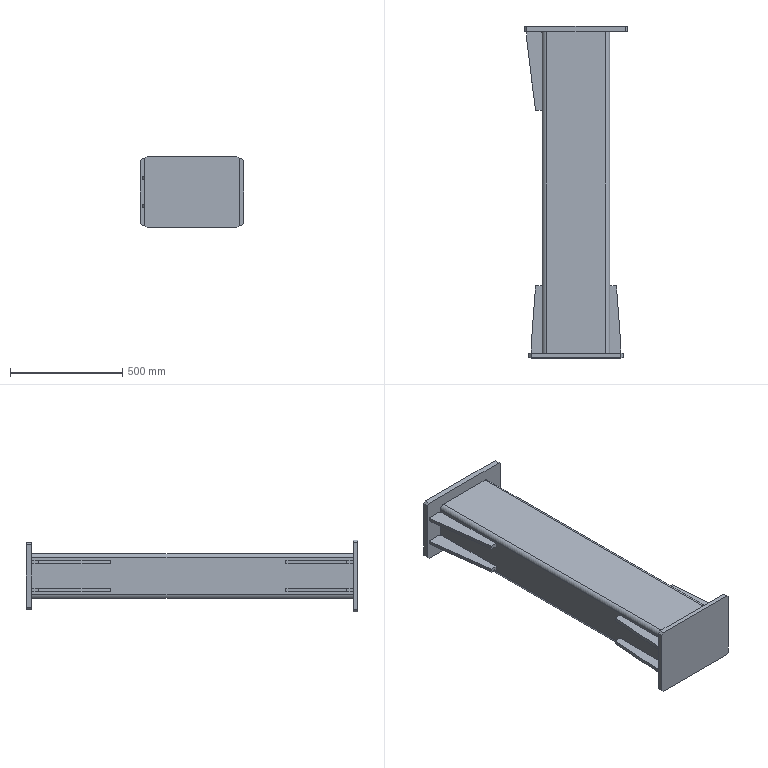Part | SolidWorks | features ICE 4, MirrorPattern 2, Extrusion 1 | 1 solid | 78 faces | box 460 x 1476 x 320 mm | volume 20749959 mm3 | plane 70 | cylinder 8 | commonest cylinder face diameters 22.142 x4 38.142 x4